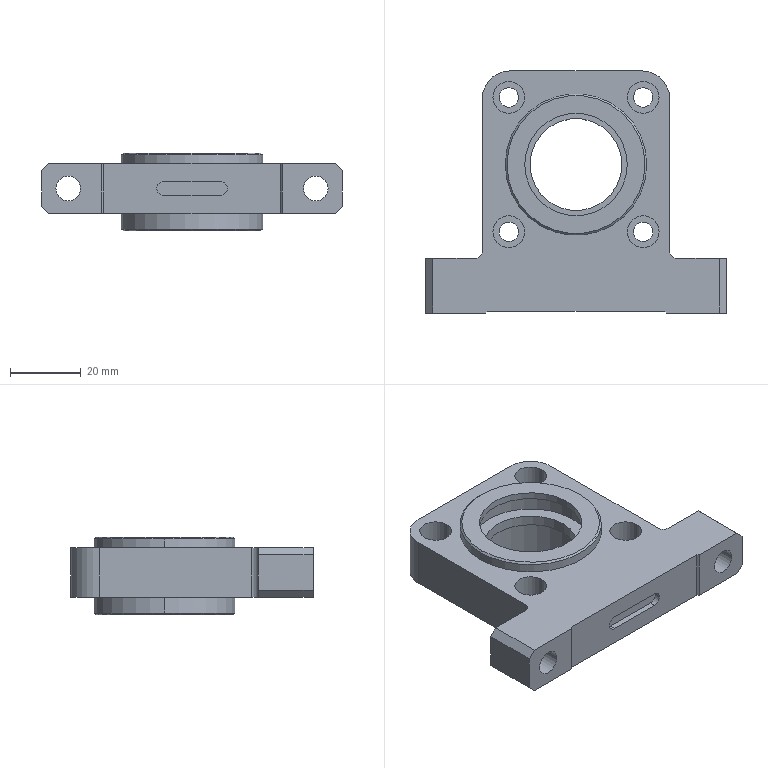Part | STEP file | 01前Flange EDA50-L_R04-001-BZ^EDA50-R04 (D60N) | 1 solid | 75 faces | box 85 x 68.5 x 22 mm | volume 45727 mm3 | cylinder 39 | plane 30 | cone 6 | commonest cylinder face diameters 5.5 x8 9 x8 4 x5 7 x4 33 x4 40 x4